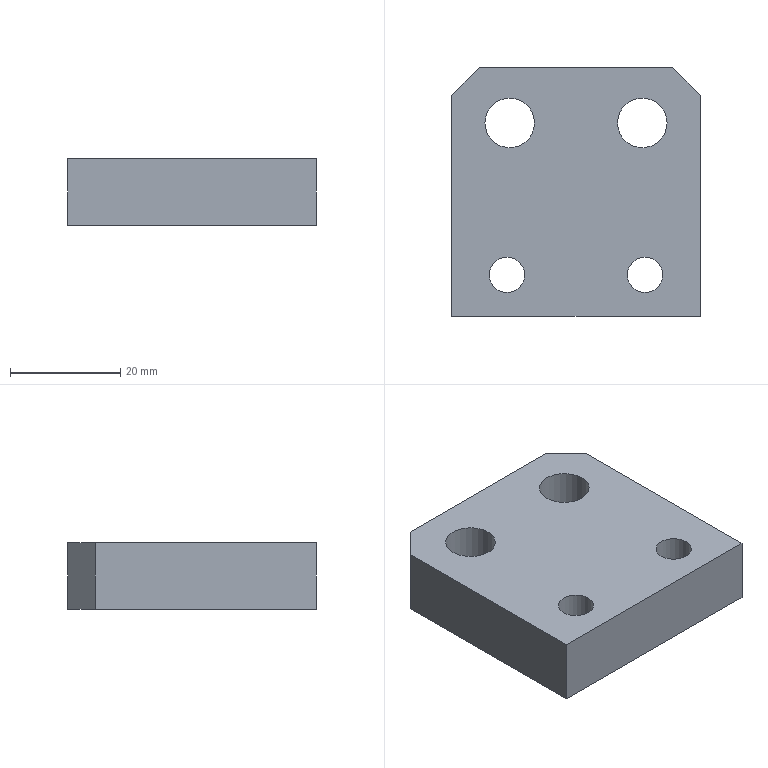Part | NX | 1 solid | 16 faces | box 45 x 45 x 12 mm | volume 20846 mm3 | plane 10 | cylinder 6 | commonest cylinder face diameters 6.4 x2 9 x2 11 x2
STEP:
#1=CARTESIAN_POINT('',(-22.5,25.,6.));
#2=VERTEX_POINT('',#1);
#3=CARTESIAN_POINT('',(-22.5,-15.,6.));
#4=VERTEX_POINT('',#3);
#5=CARTESIAN_POINT('',(-22.5,-15.,6.));
#6=DIRECTION('',(0.,-1.,0.));
#7=VECTOR('',#6,1000.);
#8=LINE('',#5,#7);
#9=EDGE_CURVE('',#2,#4,#8,.T.);
#10=ORIENTED_EDGE('',*,*,#9,.F.);
#11=CARTESIAN_POINT('',(-22.5,25.,-6.));
#12=VERTEX_POINT('',#11);
#13=CARTESIAN_POINT('',(-22.5,25.,6.));
#14=DIRECTION('',(0.,0.,-1.));
#15=VECTOR('',#14,1000.);
#16=LINE('',#13,#15);
#17=EDGE_CURVE('',#2,#12,#16,.T.);
#18=ORIENTED_EDGE('',*,*,#17,.T.);
#19=CARTESIAN_POINT('',(-22.5,-15.,-6.));
#20=VERTEX_POINT('',#19);
#21=CARTESIAN_POINT('',(-22.5,-15.,-6.));
#22=DIRECTION('',(0.,-1.,0.));
#23=VECTOR('',#22,1000.);
#24=LINE('',#21,#23);
#25=EDGE_CURVE('',#12,#20,#24,.T.);
#26=ORIENTED_EDGE('',*,*,#25,.T.);
#27=CARTESIAN_POINT('',(-22.5,-15.,6.));
#28=DIRECTION('',(0.,0.,-1.));
#29=VECTOR('',#28,1000.);
#30=LINE('',#27,#29);
#31=EDGE_CURVE('',#4,#20,#30,.T.);
#32=ORIENTED_EDGE('',*,*,#31,.F.);
#33=EDGE_LOOP('',(#10,#18,#26,#32));
#34=FACE_BOUND('',#33,.T.);
#35=CARTESIAN_POINT('',(-22.5,-15.,6.));
#36=DIRECTION('',(1.,0.,0.));
#37=DIRECTION('',(0.,1.,0.));
#38=AXIS2_PLACEMENT_3D('',#35,#36,#37);
#39=PLANE('',#38);
#40=ADVANCED_FACE('',(#34),#39,.F.);
#41=CARTESIAN_POINT('',(22.5,-15.,-6.));
#42=VERTEX_POINT('',#41);
#43=CARTESIAN_POINT('',(22.5,-15.,-6.));
#44=DIRECTION('',(1.,0.,0.));
#45=VECTOR('',#44,1000.);
#46=LINE('',#43,#45);
#47=EDGE_CURVE('',#20,#42,#46,.T.);
#48=ORIENTED_EDGE('',*,*,#47,.T.);
#49=CARTESIAN_POINT('',(22.5,-15.,6.));
#50=VERTEX_POINT('',#49);
#51=CARTESIAN_POINT('',(22.5,-15.,6.));
#52=DIRECTION('',(0.,0.,-1.));
#53=VECTOR('',#52,1000.);
#54=LINE('',#51,#53);
#55=EDGE_CURVE('',#50,#42,#54,.T.);
#56=ORIENTED_EDGE('',*,*,#55,.F.);
#57=CARTESIAN_POINT('',(22.5,-15.,6.));
#58=DIRECTION('',(1.,0.,0.));
#59=VECTOR('',#58,1000.);
#60=LINE('',#57,#59);
#61=EDGE_CURVE('',#4,#50,#60,.T.);
#62=ORIENTED_EDGE('',*,*,#61,.F.);
#63=ORIENTED_EDGE('',*,*,#31,.T.);
#64=EDGE_LOOP('',(#48,#56,#62,#63));
#65=FACE_BOUND('',#64,.T.);
#66=CARTESIAN_POINT('',(22.5,-15.,6.));
#67=DIRECTION('',(0.,1.,0.));
#68=DIRECTION('',(-1.,0.,0.));
#69=AXIS2_PLACEMENT_3D('',#66,#67,#68);
#70=PLANE('',#69);
#71=ADVANCED_FACE('',(#65),#70,.F.);
#72=CARTESIAN_POINT('',(22.5,25.,-6.));
#73=VERTEX_POINT('',#72);
#74=CARTESIAN_POINT('',(22.5,30.,-6.));
#75=DIRECTION('',(0.,1.,0.));
#76=VECTOR('',#75,1000.);
#77=LINE('',#74,#76);
#78=EDGE_CURVE('',#42,#73,#77,.T.);
#79=ORIENTED_EDGE('',*,*,#78,.T.);
#80=CARTESIAN_POINT('',(22.5,25.,6.));
#81=VERTEX_POINT('',#80);
#82=CARTESIAN_POINT('',(22.5,25.,6.));
#83=DIRECTION('',(0.,0.,1.));
#84=VECTOR('',#83,1000.);
#85=LINE('',#82,#84);
#86=EDGE_CURVE('',#73,#81,#85,.T.);
#87=ORIENTED_EDGE('',*,*,#86,.T.);
#88=CARTESIAN_POINT('',(22.5,30.,6.));
#89=DIRECTION('',(0.,1.,0.));
#90=VECTOR('',#89,1000.);
#91=LINE('',#88,#90);
#92=EDGE_CURVE('',#50,#81,#91,.T.);
#93=ORIENTED_EDGE('',*,*,#92,.F.);
#94=ORIENTED_EDGE('',*,*,#55,.T.);
#95=EDGE_LOOP('',(#79,#87,#93,#94));
#96=FACE_BOUND('',#95,.T.);
#97=CARTESIAN_POINT('',(22.5,30.,6.));
#98=DIRECTION('',(-1.,0.,0.));
#99=DIRECTION('',(0.,-1.,0.));
#100=AXIS2_PLACEMENT_3D('',#97,#98,#99);
#101=PLANE('',#100);
#102=ADVANCED_FACE('',(#96),#101,.F.);
#103=CARTESIAN_POINT('',(17.5,30.,6.));
#104=VERTEX_POINT('',#103);
#105=CARTESIAN_POINT('',(-17.5,30.,6.));
#106=VERTEX_POINT('',#105);
#107=CARTESIAN_POINT('',(-22.5,30.,6.));
#108=DIRECTION('',(-1.,0.,0.));
#109=VECTOR('',#108,1000.);
#110=LINE('',#107,#109);
#111=EDGE_CURVE('',#104,#106,#110,.T.);
#112=ORIENTED_EDGE('',*,*,#111,.F.);
#113=CARTESIAN_POINT('',(17.5,30.,-6.));
#114=VERTEX_POINT('',#113);
#115=CARTESIAN_POINT('',(17.5,30.,6.));
#116=DIRECTION('',(0.,0.,-1.));
#117=VECTOR('',#116,1000.);
#118=LINE('',#115,#117);
#119=EDGE_CURVE('',#104,#114,#118,.T.);
#120=ORIENTED_EDGE('',*,*,#119,.T.);
#121=CARTESIAN_POINT('',(-17.5,30.,-6.));
#122=VERTEX_POINT('',#121);
#123=CARTESIAN_POINT('',(-22.5,30.,-6.));
#124=DIRECTION('',(-1.,0.,0.));
#125=VECTOR('',#124,1000.);
#126=LINE('',#123,#125);
#127=EDGE_CURVE('',#114,#122,#126,.T.);
#128=ORIENTED_EDGE('',*,*,#127,.T.);
#129=CARTESIAN_POINT('',(-17.5,30.,6.));
#130=DIRECTION('',(0.,0.,1.));
#131=VECTOR('',#130,1000.);
#132=LINE('',#129,#131);
#133=EDGE_CURVE('',#122,#106,#132,.T.);
#134=ORIENTED_EDGE('',*,*,#133,.T.);
#135=EDGE_LOOP('',(#112,#120,#128,#134));
#136=FACE_BOUND('',#135,.T.);
#137=CARTESIAN_POINT('',(-22.5,30.,6.));
#138=DIRECTION('',(0.,-1.,0.));
#139=DIRECTION('',(1.,0.,0.));
#140=AXIS2_PLACEMENT_3D('',#137,#138,#139);
#141=PLANE('',#140);
#142=ADVANCED_FACE('',(#136),#141,.F.);
#143=CARTESIAN_POINT('',(-15.7,-7.5,6.));
#144=VERTEX_POINT('',#143);
#145=CARTESIAN_POINT('',(-12.5,-7.5,6.));
#146=DIRECTION('',(0.,0.,-1.));
#147=DIRECTION('',(-1.,0.,0.));
#148=AXIS2_PLACEMENT_3D('',#145,#146,#147);
#149=CIRCLE('',#148,3.2);
#150=EDGE_CURVE('',#144,#144,#149,.T.);
#151=ORIENTED_EDGE('',*,*,#150,.T.);
#152=EDGE_LOOP('',(#151));
#153=FACE_BOUND('',#152,.T.);
#154=CARTESIAN_POINT('',(9.3,-7.5,6.));
#155=VERTEX_POINT('',#154);
#156=CARTESIAN_POINT('',(12.5,-7.5,6.));
#157=DIRECTION('',(0.,0.,-1.));
#158=DIRECTION('',(-1.,0.,0.));
#159=AXIS2_PLACEMENT_3D('',#156,#157,#158);
#160=CIRCLE('',#159,3.2);
#161=EDGE_CURVE('',#155,#155,#160,.T.);
#162=ORIENTED_EDGE('',*,*,#161,.T.);
#163=EDGE_LOOP('',(#162));
#164=FACE_BOUND('',#163,.T.);
#165=CARTESIAN_POINT('',(16.5,20.,6.));
#166=VERTEX_POINT('',#165);
#167=CARTESIAN_POINT('',(12.,20.,6.));
#168=DIRECTION('',(0.,0.,1.));
#169=DIRECTION('',(1.,0.,0.));
#170=AXIS2_PLACEMENT_3D('',#167,#168,#169);
#171=CIRCLE('',#170,4.5);
#172=EDGE_CURVE('',#166,#166,#171,.T.);
#173=ORIENTED_EDGE('',*,*,#172,.F.);
#174=EDGE_LOOP('',(#173));
#175=FACE_BOUND('',#174,.T.);
#176=CARTESIAN_POINT('',(-7.5,20.,6.));
#177=VERTEX_POINT('',#176);
#178=CARTESIAN_POINT('',(-12.,20.,6.));
#179=DIRECTION('',(0.,0.,1.));
#180=DIRECTION('',(1.,0.,0.));
#181=AXIS2_PLACEMENT_3D('',#178,#179,#180);
#182=CIRCLE('',#181,4.5);
#183=EDGE_CURVE('',#177,#177,#182,.T.);
#184=ORIENTED_EDGE('',*,*,#183,.F.);
#185=EDGE_LOOP('',(#184));
#186=FACE_BOUND('',#185,.T.);
#187=ORIENTED_EDGE('',*,*,#92,.T.);
#188=CARTESIAN_POINT('',(17.5,30.,6.));
#189=DIRECTION('',(0.7071,-0.7071,0.));
#190=VECTOR('',#189,1000.);
#191=LINE('',#188,#190);
#192=EDGE_CURVE('',#81,#104,#191,.F.);
#193=ORIENTED_EDGE('',*,*,#192,.T.);
#194=ORIENTED_EDGE('',*,*,#111,.T.);
#195=CARTESIAN_POINT('',(-22.5,25.,6.));
#196=DIRECTION('',(0.7071,0.7071,0.));
#197=VECTOR('',#196,1000.);
#198=LINE('',#195,#197);
#199=EDGE_CURVE('',#106,#2,#198,.F.);
#200=ORIENTED_EDGE('',*,*,#199,.T.);
#201=ORIENTED_EDGE('',*,*,#9,.T.);
#202=ORIENTED_EDGE('',*,*,#61,.T.);
#203=EDGE_LOOP('',(#187,#193,#194,#200,#201,#202));
#204=FACE_BOUND('',#203,.T.);
#205=CARTESIAN_POINT('',(0.,0.,6.));
#206=DIRECTION('',(0.,0.,-1.));
#207=DIRECTION('',(-1.,0.,0.));
#208=AXIS2_PLACEMENT_3D('',#205,#206,#207);
#209=PLANE('',#208);
#210=ADVANCED_FACE('',(#153,#164,#175,#186,#204),#209,.F.);
#211=CARTESIAN_POINT('',(-18.,-7.5,-6.));
#212=VERTEX_POINT('',#211);
#213=CARTESIAN_POINT('',(-12.5,-7.5,-6.));
#214=DIRECTION('',(0.,0.,-1.));
#215=DIRECTION('',(-1.,0.,0.));
#216=AXIS2_PLACEMENT_3D('',#213,#214,#215);
#217=CIRCLE('',#216,5.5);
#218=EDGE_CURVE('',#212,#212,#217,.T.);
#219=ORIENTED_EDGE('',*,*,#218,.F.);
#220=EDGE_LOOP('',(#219));
#221=FACE_BOUND('',#220,.T.);
#222=CARTESIAN_POINT('',(7.,-7.5,-6.));
#223=VERTEX_POINT('',#222);
#224=CARTESIAN_POINT('',(12.5,-7.5,-6.));
#225=DIRECTION('',(0.,0.,-1.));
#226=DIRECTION('',(-1.,0.,0.));
#227=AXIS2_PLACEMENT_3D('',#224,#225,#226);
#228=CIRCLE('',#227,5.5);
#229=EDGE_CURVE('',#223,#223,#228,.T.);
#230=ORIENTED_EDGE('',*,*,#229,.F.);
#231=EDGE_LOOP('',(#230));
#232=FACE_BOUND('',#231,.T.);
#233=CARTESIAN_POINT('',(16.5,20.,-6.));
#234=VERTEX_POINT('',#233);
#235=CARTESIAN_POINT('',(12.,20.,-6.));
#236=DIRECTION('',(0.,0.,1.));
#237=DIRECTION('',(1.,0.,0.));
#238=AXIS2_PLACEMENT_3D('',#235,#236,#237);
#239=CIRCLE('',#238,4.5);
#240=EDGE_CURVE('',#234,#234,#239,.T.);
#241=ORIENTED_EDGE('',*,*,#240,.T.);
#242=EDGE_LOOP('',(#241));
#243=FACE_BOUND('',#242,.T.);
#244=CARTESIAN_POINT('',(-7.5,20.,-6.));
#245=VERTEX_POINT('',#244);
#246=CARTESIAN_POINT('',(-12.,20.,-6.));
#247=DIRECTION('',(0.,0.,1.));
#248=DIRECTION('',(1.,0.,0.));
#249=AXIS2_PLACEMENT_3D('',#246,#247,#248);
#250=CIRCLE('',#249,4.5);
#251=EDGE_CURVE('',#245,#245,#250,.T.);
#252=ORIENTED_EDGE('',*,*,#251,.T.);
#253=EDGE_LOOP('',(#252));
#254=FACE_BOUND('',#253,.T.);
#255=ORIENTED_EDGE('',*,*,#127,.F.);
#256=CARTESIAN_POINT('',(23.75,23.75,-6.));
#257=DIRECTION('',(-0.7071,0.7071,0.));
#258=VECTOR('',#257,1000.);
#259=LINE('',#256,#258);
#260=EDGE_CURVE('',#114,#73,#259,.F.);
#261=ORIENTED_EDGE('',*,*,#260,.T.);
#262=ORIENTED_EDGE('',*,*,#78,.F.);
#263=ORIENTED_EDGE('',*,*,#47,.F.);
#264=ORIENTED_EDGE('',*,*,#25,.F.);
#265=CARTESIAN_POINT('',(-23.75,23.75,-6.));
#266=DIRECTION('',(-0.7071,-0.7071,0.));
#267=VECTOR('',#266,1000.);
#268=LINE('',#265,#267);
#269=EDGE_CURVE('',#12,#122,#268,.F.);
#270=ORIENTED_EDGE('',*,*,#269,.T.);
#271=EDGE_LOOP('',(#255,#261,#262,#263,#264,#270));
#272=FACE_BOUND('',#271,.T.);
#273=CARTESIAN_POINT('',(0.,0.,-6.));
#274=DIRECTION('',(0.,0.,-1.));
#275=DIRECTION('',(-1.,0.,0.));
#276=AXIS2_PLACEMENT_3D('',#273,#274,#275);
#277=PLANE('',#276);
#278=ADVANCED_FACE('',(#221,#232,#243,#254,#272),#277,.T.);
#279=ORIENTED_EDGE('',*,*,#192,.F.);
#280=ORIENTED_EDGE('',*,*,#86,.F.);
#281=ORIENTED_EDGE('',*,*,#260,.F.);
#282=ORIENTED_EDGE('',*,*,#119,.F.);
#283=EDGE_LOOP('',(#279,#280,#281,#282));
#284=FACE_BOUND('',#283,.T.);
#285=CARTESIAN_POINT('',(17.5,30.,6.));
#286=DIRECTION('',(-0.7071,-0.7071,0.));
#287=DIRECTION('',(0.,0.,-1.));
#288=AXIS2_PLACEMENT_3D('',#285,#286,#287);
#289=PLANE('',#288);
#290=ADVANCED_FACE('',(#284),#289,.F.);
#291=ORIENTED_EDGE('',*,*,#199,.F.);
#292=ORIENTED_EDGE('',*,*,#133,.F.);
#293=ORIENTED_EDGE('',*,*,#269,.F.);
#294=ORIENTED_EDGE('',*,*,#17,.F.);
#295=EDGE_LOOP('',(#291,#292,#293,#294));
#296=FACE_BOUND('',#295,.T.);
#297=CARTESIAN_POINT('',(-22.5,25.,6.));
#298=DIRECTION('',(0.7071,-0.7071,0.));
#299=DIRECTION('',(0.,0.,-1.));
#300=AXIS2_PLACEMENT_3D('',#297,#298,#299);
#301=PLANE('',#300);
#302=ADVANCED_FACE('',(#296),#301,.F.);
#303=ORIENTED_EDGE('',*,*,#251,.F.);
#304=EDGE_LOOP('',(#303));
#305=FACE_BOUND('',#304,.T.);
#306=ORIENTED_EDGE('',*,*,#183,.T.);
#307=EDGE_LOOP('',(#306));
#308=FACE_BOUND('',#307,.T.);
#309=CARTESIAN_POINT('',(-12.,20.,6.));
#310=DIRECTION('',(0.,0.,1.));
#311=DIRECTION('',(1.,0.,0.));
#312=AXIS2_PLACEMENT_3D('',#309,#310,#311);
#313=CYLINDRICAL_SURFACE('',#312,4.5);
#314=ADVANCED_FACE('',(#305,#308),#313,.F.);
#315=ORIENTED_EDGE('',*,*,#240,.F.);
#316=EDGE_LOOP('',(#315));
#317=FACE_BOUND('',#316,.T.);
#318=ORIENTED_EDGE('',*,*,#172,.T.);
#319=EDGE_LOOP('',(#318));
#320=FACE_BOUND('',#319,.T.);
#321=CARTESIAN_POINT('',(12.,20.,6.));
#322=DIRECTION('',(0.,0.,1.));
#323=DIRECTION('',(1.,0.,0.));
#324=AXIS2_PLACEMENT_3D('',#321,#322,#323);
#325=CYLINDRICAL_SURFACE('',#324,4.5);
#326=ADVANCED_FACE('',(#317,#320),#325,.F.);
#327=ORIENTED_EDGE('',*,*,#161,.F.);
#328=EDGE_LOOP('',(#327));
#329=FACE_BOUND('',#328,.T.);
#330=CARTESIAN_POINT('',(9.3,-7.5,0.8));
#331=VERTEX_POINT('',#330);
#332=CARTESIAN_POINT('',(12.5,-7.5,0.8));
#333=DIRECTION('',(0.,0.,-1.));
#334=DIRECTION('',(-1.,0.,0.));
#335=AXIS2_PLACEMENT_3D('',#332,#333,#334);
#336=CIRCLE('',#335,3.2);
#337=EDGE_CURVE('',#331,#331,#336,.T.);
#338=ORIENTED_EDGE('',*,*,#337,.T.);
#339=EDGE_LOOP('',(#338));
#340=FACE_BOUND('',#339,.T.);
#341=CARTESIAN_POINT('',(12.5,-7.5,-6.));
#342=DIRECTION('',(0.,0.,-1.));
#343=DIRECTION('',(-1.,0.,0.));
#344=AXIS2_PLACEMENT_3D('',#341,#342,#343);
#345=CYLINDRICAL_SURFACE('',#344,3.2);
#346=ADVANCED_FACE('',(#329,#340),#345,.F.);
#347=ORIENTED_EDGE('',*,*,#337,.F.);
#348=EDGE_LOOP('',(#347));
#349=FACE_BOUND('',#348,.T.);
#350=CARTESIAN_POINT('',(7.,-7.5,0.8));
#351=VERTEX_POINT('',#350);
#352=CARTESIAN_POINT('',(12.5,-7.5,0.8));
#353=DIRECTION('',(0.,0.,-1.));
#354=DIRECTION('',(-1.,0.,0.));
#355=AXIS2_PLACEMENT_3D('',#352,#353,#354);
#356=CIRCLE('',#355,5.5);
#357=EDGE_CURVE('',#351,#351,#356,.T.);
#358=ORIENTED_EDGE('',*,*,#357,.T.);
#359=EDGE_LOOP('',(#358));
#360=FACE_BOUND('',#359,.T.);
#361=CARTESIAN_POINT('',(15.7,-7.5,0.8));
#362=DIRECTION('',(0.,0.,1.));
#363=DIRECTION('',(1.,0.,0.));
#364=AXIS2_PLACEMENT_3D('',#361,#362,#363);
#365=PLANE('',#364);
#366=ADVANCED_FACE('',(#349,#360),#365,.F.);
#367=ORIENTED_EDGE('',*,*,#357,.F.);
#368=EDGE_LOOP('',(#367));
#369=FACE_BOUND('',#368,.T.);
#370=ORIENTED_EDGE('',*,*,#229,.T.);
#371=EDGE_LOOP('',(#370));
#372=FACE_BOUND('',#371,.T.);
#373=CARTESIAN_POINT('',(12.5,-7.5,-6.));
#374=DIRECTION('',(0.,0.,-1.));
#375=DIRECTION('',(-1.,0.,0.));
#376=AXIS2_PLACEMENT_3D('',#373,#374,#375);
#377=CYLINDRICAL_SURFACE('',#376,5.5);
#378=ADVANCED_FACE('',(#369,#372),#377,.F.);
#379=ORIENTED_EDGE('',*,*,#150,.F.);
#380=EDGE_LOOP('',(#379));
#381=FACE_BOUND('',#380,.T.);
#382=CARTESIAN_POINT('',(-15.7,-7.5,0.8));
#383=VERTEX_POINT('',#382);
#384=CARTESIAN_POINT('',(-12.5,-7.5,0.8));
#385=DIRECTION('',(0.,0.,-1.));
#386=DIRECTION('',(-1.,0.,0.));
#387=AXIS2_PLACEMENT_3D('',#384,#385,#386);
#388=CIRCLE('',#387,3.2);
#389=EDGE_CURVE('',#383,#383,#388,.T.);
#390=ORIENTED_EDGE('',*,*,#389,.T.);
#391=EDGE_LOOP('',(#390));
#392=FACE_BOUND('',#391,.T.);
#393=CARTESIAN_POINT('',(-12.5,-7.5,-6.));
#394=DIRECTION('',(0.,0.,-1.));
#395=DIRECTION('',(-1.,0.,0.));
#396=AXIS2_PLACEMENT_3D('',#393,#394,#395);
#397=CYLINDRICAL_SURFACE('',#396,3.2);
#398=ADVANCED_FACE('',(#381,#392),#397,.F.);
#399=ORIENTED_EDGE('',*,*,#389,.F.);
#400=EDGE_LOOP('',(#399));
#401=FACE_BOUND('',#400,.T.);
#402=CARTESIAN_POINT('',(-18.,-7.5,0.8));
#403=VERTEX_POINT('',#402);
#404=CARTESIAN_POINT('',(-12.5,-7.5,0.8));
#405=DIRECTION('',(0.,0.,-1.));
#406=DIRECTION('',(-1.,0.,0.));
#407=AXIS2_PLACEMENT_3D('',#404,#405,#406);
#408=CIRCLE('',#407,5.5);
#409=EDGE_CURVE('',#403,#403,#408,.T.);
#410=ORIENTED_EDGE('',*,*,#409,.T.);
#411=EDGE_LOOP('',(#410));
#412=FACE_BOUND('',#411,.T.);
#413=CARTESIAN_POINT('',(-9.3,-7.5,0.8));
#414=DIRECTION('',(0.,0.,1.));
#415=DIRECTION('',(1.,0.,0.));
#416=AXIS2_PLACEMENT_3D('',#413,#414,#415);
#417=PLANE('',#416);
#418=ADVANCED_FACE('',(#401,#412),#417,.F.);
#419=ORIENTED_EDGE('',*,*,#409,.F.);
#420=EDGE_LOOP('',(#419));
#421=FACE_BOUND('',#420,.T.);
#422=ORIENTED_EDGE('',*,*,#218,.T.);
#423=EDGE_LOOP('',(#422));
#424=FACE_BOUND('',#423,.T.);
#425=CARTESIAN_POINT('',(-12.5,-7.5,-6.));
#426=DIRECTION('',(0.,0.,-1.));
#427=DIRECTION('',(-1.,0.,0.));
#428=AXIS2_PLACEMENT_3D('',#425,#426,#427);
#429=CYLINDRICAL_SURFACE('',#428,5.5);
#430=ADVANCED_FACE('',(#421,#424),#429,.F.);
#431=CLOSED_SHELL('',(#40,#71,#102,#142,#210,#278,#290,#302,#314,#326,#346,#366,#378,#398,#418,#430));
#432=MANIFOLD_SOLID_BREP('',#431);
#433=(LENGTH_UNIT()NAMED_UNIT(*)SI_UNIT(.MILLI.,.METRE.));
#434=UNCERTAINTY_MEASURE_WITH_UNIT(LENGTH_MEASURE(0.00001),#433,'','');
#435=(NAMED_UNIT(*)PLANE_ANGLE_UNIT()SI_UNIT($,.RADIAN.));
#436=(NAMED_UNIT(*)SI_UNIT($,.STERADIAN.)SOLID_ANGLE_UNIT());
#437=(GEOMETRIC_REPRESENTATION_CONTEXT(3)GLOBAL_UNCERTAINTY_ASSIGNED_CONTEXT((#434))GLOBAL_UNIT_ASSIGNED_CONTEXT((#433,#435,#436))REPRESENTATION_CONTEXT('',''));
#438=ADVANCED_BREP_SHAPE_REPRESENTATION('',(#432),#437);